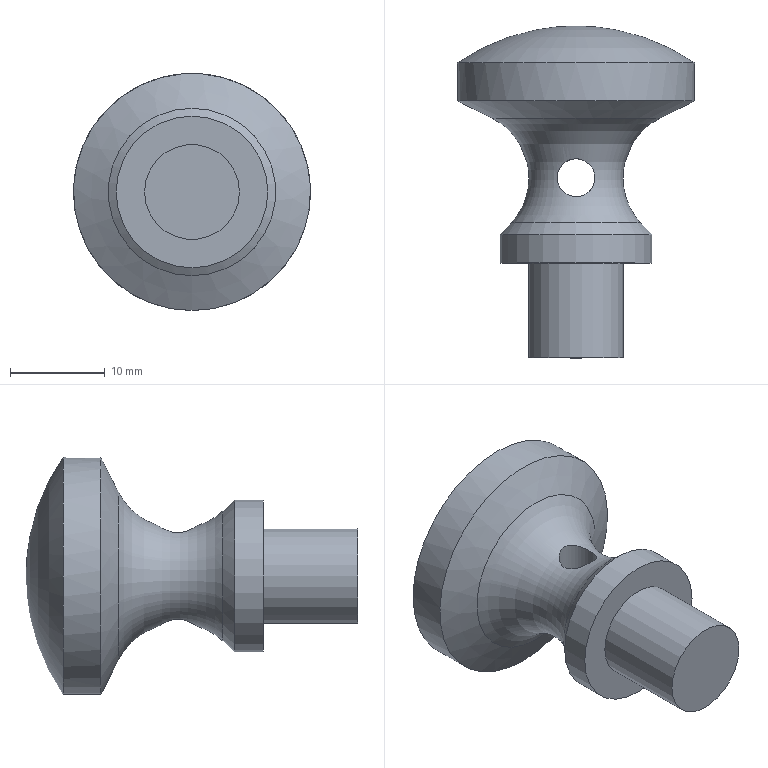Part | NX | features DATUM_CSYS 5, SKETCH 4, EXTRUDE 3, SWP104 1 | 3 solids | 13 faces | box 25 x 35 x 25 mm | volume 6314 mm3 | plane 5 | cylinder 4 | torus 2 | cone 2 | commonest cylinder face diameters 4 x1 10 x1 16 x1 25 x1
STEP:
#1=CARTESIAN_POINT('',(8.,3.,0.));
#2=VERTEX_POINT('',#1);
#3=CARTESIAN_POINT('',(0.,3.,0.));
#4=DIRECTION('',(0.,-1.,0.));
#5=DIRECTION('',(1.,0.,0.));
#6=AXIS2_PLACEMENT_3D('',#3,#4,#5);
#7=CIRCLE('',#6,8.);
#8=EDGE_CURVE('',#2,#2,#7,.T.);
#9=ORIENTED_EDGE('',*,*,#8,.T.);
#10=EDGE_LOOP('',(#9));
#11=FACE_BOUND('',#10,.T.);
#12=CARTESIAN_POINT('',(8.,0.,0.));
#13=VERTEX_POINT('',#12);
#14=CARTESIAN_POINT('',(0.,0.,0.));
#15=DIRECTION('',(0.,-1.,0.));
#16=DIRECTION('',(1.,0.,0.));
#17=AXIS2_PLACEMENT_3D('',#14,#15,#16);
#18=CIRCLE('',#17,8.);
#19=EDGE_CURVE('',#13,#13,#18,.T.);
#20=ORIENTED_EDGE('',*,*,#19,.F.);
#21=EDGE_LOOP('',(#20));
#22=FACE_BOUND('',#21,.T.);
#23=CARTESIAN_POINT('',(0.,3.,0.));
#24=DIRECTION('',(0.,-1.,0.));
#25=DIRECTION('',(0.,0.,-1.));
#26=AXIS2_PLACEMENT_3D('',#23,#24,#25);
#27=CYLINDRICAL_SURFACE('',#26,8.);
#28=ADVANCED_FACE('',(#11,#22),#27,.T.);
#29=ORIENTED_EDGE('',*,*,#8,.F.);
#30=EDGE_LOOP('',(#29));
#31=FACE_BOUND('',#30,.T.);
#32=CARTESIAN_POINT('',(0.,3.,0.));
#33=DIRECTION('',(0.,-1.,0.));
#34=DIRECTION('',(0.,0.,-1.));
#35=AXIS2_PLACEMENT_3D('',#32,#33,#34);
#36=PLANE('',#35);
#37=ADVANCED_FACE('',(#31),#36,.F.);
#38=ORIENTED_EDGE('',*,*,#19,.T.);
#39=EDGE_LOOP('',(#38));
#40=FACE_BOUND('',#39,.T.);
#41=CARTESIAN_POINT('',(0.,0.,0.));
#42=DIRECTION('',(0.,-1.,0.));
#43=DIRECTION('',(0.,0.,-1.));
#44=AXIS2_PLACEMENT_3D('',#41,#42,#43);
#45=PLANE('',#44);
#46=ADVANCED_FACE('',(#40),#45,.T.);
#47=CLOSED_SHELL('',(#28,#37,#46));
#48=MANIFOLD_SOLID_BREP('',#47);
#49=CARTESIAN_POINT('',(-1.448,7.62,4.909));
#50=VERTEX_POINT('',#49);
#51=CARTESIAN_POINT('',(-0.04497,6.782,5.442));
#52=CARTESIAN_POINT('',(-1.607,7.473,4.909));
#53=CARTESIAN_POINT('',(-2.213,9.049,4.377));
#54=CARTESIAN_POINT('',(-1.537,10.597,4.956));
#55=CARTESIAN_POINT('',(0.04697,11.217,5.442));
#56=CARTESIAN_POINT('',(1.601,10.532,4.912));
#57=CARTESIAN_POINT('',(2.215,8.954,4.376));
#58=CARTESIAN_POINT('',(1.535,7.402,4.956));
#59=CARTESIAN_POINT('',(-0.04497,6.782,5.442));
#60=CARTESIAN_POINT('',(-1.607,7.473,4.909));
#61=CARTESIAN_POINT('',(-2.213,9.049,4.377));
#62=B_SPLINE_CURVE_WITH_KNOTS('',3,(#51,#52,#53,#54,#55,#56,#57,#58,#59,#60,#61),.UNSPECIFIED.,.T.,.F.,(1,1,1,1,1,1,1,1,1,1,1,1,1,1,1),(-0.004826,-0.003217,-0.001609,0.,0.001609,0.003217,0.004826,0.006435,0.008043,0.009652,0.01126,0.01287,0.01448,0.01609,0.0177),.UNSPECIFIED.);
#63=EDGE_CURVE('',#50,#50,#62,.T.);
#64=ORIENTED_EDGE('',*,*,#63,.T.);
#65=EDGE_LOOP('',(#64));
#66=FACE_BOUND('',#65,.T.);
#67=CARTESIAN_POINT('',(0.,15.251,-8.831));
#68=VERTEX_POINT('',#67);
#69=CARTESIAN_POINT('',(0.,15.251,0.));
#70=DIRECTION('',(0.,-1.,0.));
#71=DIRECTION('',(0.,0.,-1.));
#72=AXIS2_PLACEMENT_3D('',#69,#70,#71);
#73=CIRCLE('',#72,8.831);
#74=EDGE_CURVE('',#68,#68,#73,.T.);
#75=ORIENTED_EDGE('',*,*,#74,.T.);
#76=EDGE_LOOP('',(#75));
#77=FACE_BOUND('',#76,.T.);
#78=CARTESIAN_POINT('',(0.,4.236,-6.852));
#79=VERTEX_POINT('',#78);
#80=CARTESIAN_POINT('',(0.,4.236,0.));
#81=DIRECTION('',(0.,-1.,0.));
#82=DIRECTION('',(0.,0.,-1.));
#83=AXIS2_PLACEMENT_3D('',#80,#81,#82);
#84=CIRCLE('',#83,6.852);
#85=EDGE_CURVE('',#79,#79,#84,.T.);
#86=ORIENTED_EDGE('',*,*,#85,.F.);
#87=EDGE_LOOP('',(#86));
#88=FACE_BOUND('',#87,.T.);
#89=CARTESIAN_POINT('',(-1.233,7.426,-5.011));
#90=VERTEX_POINT('',#89);
#91=CARTESIAN_POINT('',(-2.198,8.713,-4.394));
#92=CARTESIAN_POINT('',(-1.373,7.26,-5.061));
#93=CARTESIAN_POINT('',(0.2879,6.802,-5.426));
#94=CARTESIAN_POINT('',(1.741,7.629,-4.806));
#95=CARTESIAN_POINT('',(2.197,9.284,-4.394));
#96=CARTESIAN_POINT('',(1.378,10.736,-5.058));
#97=CARTESIAN_POINT('',(-0.2854,11.199,-5.427));
#98=CARTESIAN_POINT('',(-1.74,10.373,-4.806));
#99=CARTESIAN_POINT('',(-2.198,8.713,-4.394));
#100=CARTESIAN_POINT('',(-1.373,7.26,-5.061));
#101=CARTESIAN_POINT('',(0.2879,6.802,-5.426));
#102=B_SPLINE_CURVE_WITH_KNOTS('',3,(#91,#92,#93,#94,#95,#96,#97,#98,#99,#100,#101),.UNSPECIFIED.,.T.,.F.,(1,1,1,1,1,1,1,1,1,1,1,1,1,1,1),(-0.00483,-0.00322,-0.00161,0.,0.00161,0.00322,0.00483,0.00644,0.008049,0.009659,0.01127,0.01288,0.01449,0.0161,0.01771),.UNSPECIFIED.);
#103=EDGE_CURVE('',#90,#90,#102,.T.);
#104=ORIENTED_EDGE('',*,*,#103,.T.);
#105=EDGE_LOOP('',(#104));
#106=FACE_BOUND('',#105,.T.);
#107=CARTESIAN_POINT('',(0.,9.,0.));
#108=DIRECTION('',(0.,-1.,0.));
#109=DIRECTION('',(0.,0.,-1.));
#110=AXIS2_PLACEMENT_3D('',#107,#108,#109);
#111=TOROIDAL_SURFACE('',#110,11.981,7.);
#112=ADVANCED_FACE('',(#66,#77,#88,#106),#111,.F.);
#113=CARTESIAN_POINT('',(0.,3.,-8.));
#114=VERTEX_POINT('',#113);
#115=CARTESIAN_POINT('',(0.,3.,0.));
#116=DIRECTION('',(0.,-1.,0.));
#117=DIRECTION('',(0.,0.,-1.));
#118=AXIS2_PLACEMENT_3D('',#115,#116,#117);
#119=CIRCLE('',#118,8.);
#120=EDGE_CURVE('',#114,#114,#119,.T.);
#121=ORIENTED_EDGE('',*,*,#120,.T.);
#122=EDGE_LOOP('',(#121));
#123=FACE_BOUND('',#122,.T.);
#124=CARTESIAN_POINT('',(0.,3.,0.));
#125=DIRECTION('',(0.,-1.,0.));
#126=DIRECTION('',(0.,0.,-1.));
#127=AXIS2_PLACEMENT_3D('',#124,#125,#126);
#128=PLANE('',#127);
#129=ADVANCED_FACE('',(#123),#128,.T.);
#130=ORIENTED_EDGE('',*,*,#85,.T.);
#131=EDGE_LOOP('',(#130));
#132=FACE_BOUND('',#131,.T.);
#133=ORIENTED_EDGE('',*,*,#120,.F.);
#134=EDGE_LOOP('',(#133));
#135=FACE_BOUND('',#134,.T.);
#136=CARTESIAN_POINT('',(0.,3.,0.));
#137=DIRECTION('',(0.,-1.,0.));
#138=DIRECTION('',(0.,0.,-1.));
#139=AXIS2_PLACEMENT_3D('',#136,#137,#138);
#140=CONICAL_SURFACE('',#139,8.,0.7485);
#141=ADVANCED_FACE('',(#132,#135),#140,.T.);
#142=CARTESIAN_POINT('',(0.,17.1,-12.5));
#143=VERTEX_POINT('',#142);
#144=CARTESIAN_POINT('',(0.,17.1,0.));
#145=DIRECTION('',(0.,-1.,0.));
#146=DIRECTION('',(0.,0.,-1.));
#147=AXIS2_PLACEMENT_3D('',#144,#145,#146);
#148=CIRCLE('',#147,12.5);
#149=EDGE_CURVE('',#143,#143,#148,.T.);
#150=ORIENTED_EDGE('',*,*,#149,.T.);
#151=EDGE_LOOP('',(#150));
#152=FACE_BOUND('',#151,.T.);
#153=ORIENTED_EDGE('',*,*,#74,.F.);
#154=EDGE_LOOP('',(#153));
#155=FACE_BOUND('',#154,.T.);
#156=CARTESIAN_POINT('',(0.,15.251,0.));
#157=DIRECTION('',(0.,1.,0.));
#158=DIRECTION('',(0.,0.,1.));
#159=AXIS2_PLACEMENT_3D('',#156,#157,#158);
#160=CONICAL_SURFACE('',#159,8.831,1.104);
#161=ADVANCED_FACE('',(#152,#155),#160,.T.);
#162=CARTESIAN_POINT('',(0.,21.1,-12.5));
#163=VERTEX_POINT('',#162);
#164=CARTESIAN_POINT('',(0.,21.1,0.));
#165=DIRECTION('',(0.,-1.,0.));
#166=DIRECTION('',(0.,0.,-1.));
#167=AXIS2_PLACEMENT_3D('',#164,#165,#166);
#168=CIRCLE('',#167,12.5);
#169=EDGE_CURVE('',#163,#163,#168,.T.);
#170=ORIENTED_EDGE('',*,*,#169,.T.);
#171=EDGE_LOOP('',(#170));
#172=FACE_BOUND('',#171,.T.);
#173=ORIENTED_EDGE('',*,*,#149,.F.);
#174=EDGE_LOOP('',(#173));
#175=FACE_BOUND('',#174,.T.);
#176=CARTESIAN_POINT('',(0.,-10.,0.));
#177=DIRECTION('',(0.,-1.,0.));
#178=DIRECTION('',(0.,0.,-1.));
#179=AXIS2_PLACEMENT_3D('',#176,#177,#178);
#180=CYLINDRICAL_SURFACE('',#179,12.5);
#181=ADVANCED_FACE('',(#172,#175),#180,.T.);
#182=CARTESIAN_POINT('',(0.,25.,0.));
#183=VERTEX_POINT('',#182);
#184=VERTEX_LOOP('',#183);
#185=FACE_BOUND('',#184,.T.);
#186=ORIENTED_EDGE('',*,*,#169,.F.);
#187=EDGE_LOOP('',(#186));
#188=FACE_BOUND('',#187,.T.);
#189=CARTESIAN_POINT('',(0.,3.,0.));
#190=DIRECTION('',(0.,-1.,0.));
#191=DIRECTION('',(0.,0.,-1.));
#192=AXIS2_PLACEMENT_3D('',#189,#190,#191);
#193=DEGENERATE_TOROIDAL_SURFACE('',#192,0.0056,22.,.F.);
#194=ADVANCED_FACE('',(#185,#188),#193,.F.);
#195=ORIENTED_EDGE('',*,*,#103,.F.);
#196=EDGE_LOOP('',(#195));
#197=FACE_BOUND('',#196,.T.);
#198=ORIENTED_EDGE('',*,*,#63,.F.);
#199=EDGE_LOOP('',(#198));
#200=FACE_BOUND('',#199,.T.);
#201=CARTESIAN_POINT('',(0.,9.,8.5));
#202=DIRECTION('',(0.,0.,-1.));
#203=DIRECTION('',(-1.,0.,0.));
#204=AXIS2_PLACEMENT_3D('',#201,#202,#203);
#205=CYLINDRICAL_SURFACE('',#204,2.);
#206=ADVANCED_FACE('',(#197,#200),#205,.F.);
#207=CLOSED_SHELL('',(#112,#129,#141,#161,#181,#194,#206));
#208=MANIFOLD_SOLID_BREP('',#207);
#209=CARTESIAN_POINT('',(5.,-10.,0.));
#210=VERTEX_POINT('',#209);
#211=CARTESIAN_POINT('',(0.,-10.,0.));
#212=DIRECTION('',(0.,-1.,0.));
#213=DIRECTION('',(1.,0.,0.));
#214=AXIS2_PLACEMENT_3D('',#211,#212,#213);
#215=CIRCLE('',#214,5.);
#216=EDGE_CURVE('',#210,#210,#215,.T.);
#217=ORIENTED_EDGE('',*,*,#216,.F.);
#218=EDGE_LOOP('',(#217));
#219=FACE_BOUND('',#218,.T.);
#220=CARTESIAN_POINT('',(5.,0.,0.));
#221=VERTEX_POINT('',#220);
#222=CARTESIAN_POINT('',(0.,0.,0.));
#223=DIRECTION('',(0.,-1.,0.));
#224=DIRECTION('',(1.,0.,0.));
#225=AXIS2_PLACEMENT_3D('',#222,#223,#224);
#226=CIRCLE('',#225,5.);
#227=EDGE_CURVE('',#221,#221,#226,.T.);
#228=ORIENTED_EDGE('',*,*,#227,.T.);
#229=EDGE_LOOP('',(#228));
#230=FACE_BOUND('',#229,.T.);
#231=CARTESIAN_POINT('',(0.,-10.,0.));
#232=DIRECTION('',(0.,1.,0.));
#233=DIRECTION('',(0.,0.,1.));
#234=AXIS2_PLACEMENT_3D('',#231,#232,#233);
#235=CYLINDRICAL_SURFACE('',#234,5.);
#236=ADVANCED_FACE('',(#219,#230),#235,.T.);
#237=ORIENTED_EDGE('',*,*,#216,.T.);
#238=EDGE_LOOP('',(#237));
#239=FACE_BOUND('',#238,.T.);
#240=CARTESIAN_POINT('',(0.,-10.,0.));
#241=DIRECTION('',(0.,-1.,0.));
#242=DIRECTION('',(0.,0.,-1.));
#243=AXIS2_PLACEMENT_3D('',#240,#241,#242);
#244=PLANE('',#243);
#245=ADVANCED_FACE('',(#239),#244,.T.);
#246=ORIENTED_EDGE('',*,*,#227,.F.);
#247=EDGE_LOOP('',(#246));
#248=FACE_BOUND('',#247,.T.);
#249=CARTESIAN_POINT('',(0.,0.,0.));
#250=DIRECTION('',(0.,-1.,0.));
#251=DIRECTION('',(0.,0.,-1.));
#252=AXIS2_PLACEMENT_3D('',#249,#250,#251);
#253=PLANE('',#252);
#254=ADVANCED_FACE('',(#248),#253,.F.);
#255=CLOSED_SHELL('',(#236,#245,#254));
#256=MANIFOLD_SOLID_BREP('',#255);
#257=(LENGTH_UNIT()NAMED_UNIT(*)SI_UNIT(.MILLI.,.METRE.));
#258=UNCERTAINTY_MEASURE_WITH_UNIT(LENGTH_MEASURE(0.0508),#257,'','');
#259=(NAMED_UNIT(*)PLANE_ANGLE_UNIT()SI_UNIT($,.RADIAN.));
#260=(NAMED_UNIT(*)SI_UNIT($,.STERADIAN.)SOLID_ANGLE_UNIT());
#261=(GEOMETRIC_REPRESENTATION_CONTEXT(3)GLOBAL_UNCERTAINTY_ASSIGNED_CONTEXT((#258))GLOBAL_UNIT_ASSIGNED_CONTEXT((#257,#259,#260))REPRESENTATION_CONTEXT('',''));
#262=ADVANCED_BREP_SHAPE_REPRESENTATION('',(#48,#208,#256),#261);